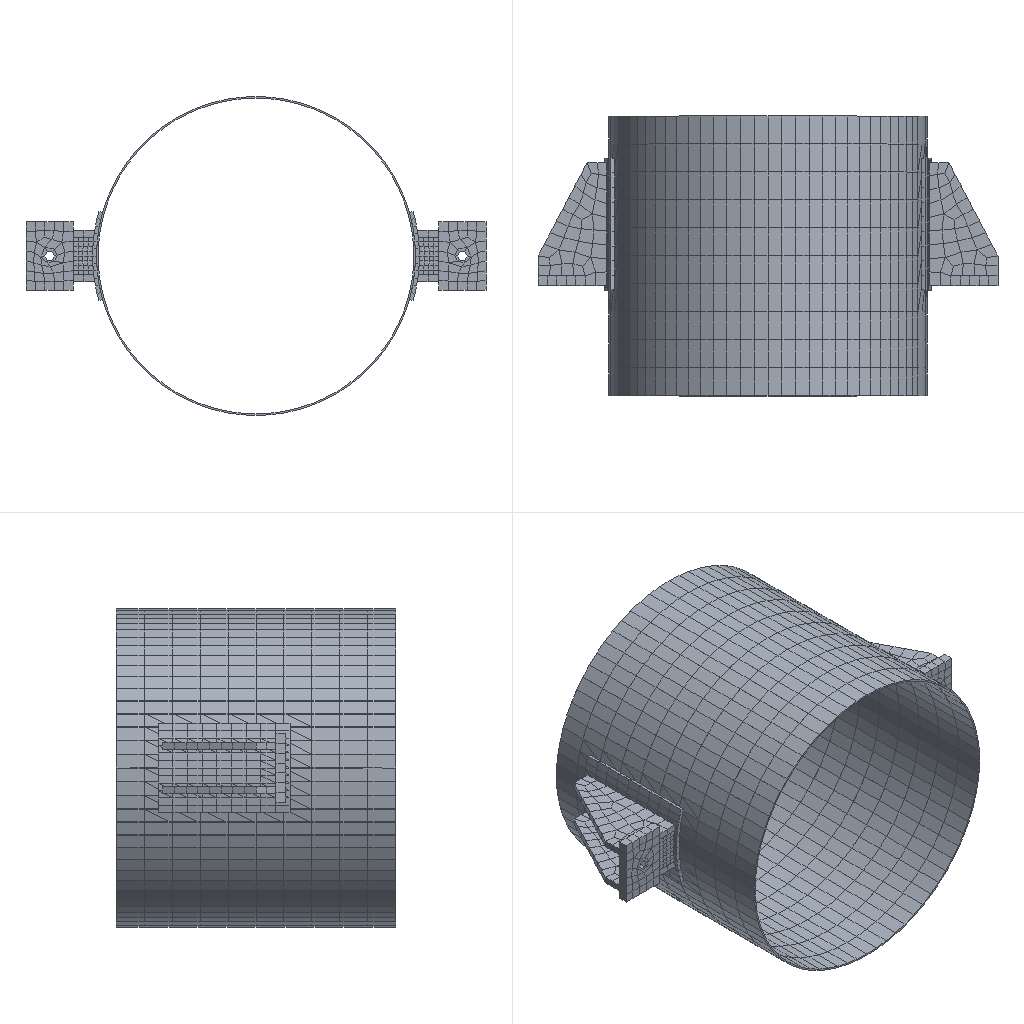Simulation study | ansys workbench
Ansys APDL input file, long lists of numbers shortened:
/batch
/config,noeldb,1     ! force off writing results to database
*get,_wallstrt,active,,time,wall
! ANSYS input file written by Workbench version 2022 R1
! File used for geometry attach:
/title,wbnew--____ (C5)
! ****** Begin Custom Load Command Snippet ******
/COM, ACT Extensions:
/COM,     LSDYNA, 2021.1
/COM,
! ****** End   Custom Load Command Snippet ******
*DIM,_wb_ProjectScratch_dir,string,248
_wb_ProjectScratch_dir(1) = ''
*DIM,_wb_SolverFiles_dir,string,248
_wb_SolverFiles_dir(1) = ''
*DIM,_wb_userfiles_dir,string,248
_wb_userfiles_dir(1) = ''
/com,--- Data in consistent NMM units. See Solving Units in the help system for more information.
/units,MPA
/nopr
/wb,file,start              !  signify a WB generated input file
/prep7
! Turn off shape checking because checks already performed inside WB mesher.
! See help system for more information.
SHPP,OFF,,NOWARN
/nolist
etcon,set             ! allow ANSYS to choose best KEYOP's for 180x elements, resets any applicable keyopt to MAPDL defaults
/com,*********** Nodes for the whole assembly ***********
nblock,3,,11156
(1i9,3e20.9e3)
        1    -9.929159159E+02     6.715040761E+02    -9.500000000E+01
! (10141 more lines like these left out)
-1
/wb,elem,start            !  set before creation of elements
/com,*********** Elements for Body 1 "__1^___1|__-__1" ***********
et,1,186
keyo,1,2,1          ! set full integration on SOLID186
eblock,19,solid,,720
(19i9)
        1        1        1        1        0        0        0        0       20        0      583     5200     5908     5907     5201     5204     5943     5942     5202
! (1439 more lines like these left out)
-1
/com,*********** Elements for Body 2 "__2^___1|__-__1" ***********
et,2,186
keyo,2,2,1          ! set full integration on SOLID186
eblock,19,solid,,108
(19i9)
        2        2        2        2        0        0        0        0       20        0      394     3257     3307     3371     3379     3293     3294     3370     3423
! (215 more lines like these left out)
-1
/com,*********** Elements for Body 3 "__3^___1|__-__1" ***********
et,3,186
keyo,3,2,1          ! set full integration on SOLID186
eblock,19,solid,,43
(19i9)
        3        3        3        3        0        0        0        0       20        0      103      797      820      801      798      844      821      840      843
! (85 more lines like these left out)
-1
/com,*********** Elements for Body 4 "__4^___1|__-__1" ***********
et,4,186
keyo,4,2,1          ! set full integration on SOLID186
eblock,19,solid,,38
(19i9)
        4        4        4        4        0        0        0        0       20        0      210     1631     1642     1646     1636     1662     1651     1647     1657
! (75 more lines like these left out)
-1
/com,*********** Elements for Body 5 "__4^___1|__-__1[2]" ***********
et,5,186
keyo,5,2,1          ! set full integration on SOLID186
eblock,19,solid,,38
(19i9)
        5        5        5        5        0        0        0        0       20        0      356     2834     2845     2849     2839     2865     2854     2850     2860
! (75 more lines like these left out)
-1
! (6 more sections like these left out)
/wb,elem,end               !  done creating elements
/com,*********** Send User Defined Coordinate System(s) ***********
csys,0
toffst,273.15,  ! Temperature offset from absolute zero
/com,*********** Set Reference Temperature ***********
tref,22.
/wb,mat,start              !  starting to send materials
/com,*********** Send Materials ***********
Temperature = 'TEMP' ! Temperature
MP,DENS,1,7.85e-09,	! tonne mm^-3
MP,ALPX,1,1.2e-05,	! C^-1
MP,C,1,434000000,	! mm^2 s^-2 C^-1
MP,KXX,1,60.5,	! tonne mm s^-3 C^-1
MP,RSVX,1,0.00017,	! ohm mm
MP,EX,1,200000,	! tonne s^-2 mm^-1
MP,NUXY,1,0.3,
MP,MURX,1,10000,
Temperature = 'TEMP' ! Temperature
MP,DENS,2,7.85e-09,	! tonne mm^-3
MP,ALPX,2,1.2e-05,	! C^-1
MP,C,2,434000000,	! mm^2 s^-2 C^-1
MP,KXX,2,60.5,	! tonne mm s^-3 C^-1
MP,RSVX,2,0.00017,	! ohm mm
MP,EX,2,200000,	! tonne s^-2 mm^-1
MP,NUXY,2,0.3,
MP,MURX,2,10000,
Temperature = 'TEMP' ! Temperature
MP,DENS,3,7.85e-09,	! tonne mm^-3
MP,ALPX,3,1.2e-05,	! C^-1
MP,C,3,434000000,	! mm^2 s^-2 C^-1
MP,KXX,3,60.5,	! tonne mm s^-3 C^-1
MP,RSVX,3,0.00017,	! ohm mm
MP,EX,3,200000,	! tonne s^-2 mm^-1
MP,NUXY,3,0.3,
MP,MURX,3,10000,
Temperature = 'TEMP' ! Temperature
MP,DENS,4,7.85e-09,	! tonne mm^-3
MP,ALPX,4,1.2e-05,	! C^-1
MP,C,4,434000000,	! mm^2 s^-2 C^-1
MP,KXX,4,60.5,	! tonne mm s^-3 C^-1
MP,RSVX,4,0.00017,	! ohm mm
MP,EX,4,200000,	! tonne s^-2 mm^-1
MP,NUXY,4,0.3,
MP,MURX,4,10000,
Temperature = 'TEMP' ! Temperature
MP,DENS,5,7.85e-09,	! tonne mm^-3
MP,ALPX,5,1.2e-05,	! C^-1
MP,C,5,434000000,	! mm^2 s^-2 C^-1
MP,KXX,5,60.5,	! tonne mm s^-3 C^-1
MP,RSVX,5,0.00017,	! ohm mm
MP,EX,5,200000,	! tonne s^-2 mm^-1
MP,NUXY,5,0.3,
MP,MURX,5,10000,
Temperature = 'TEMP' ! Temperature
MP,DENS,6,7.85e-09,	! tonne mm^-3
MP,ALPX,6,1.2e-05,	! C^-1
MP,C,6,434000000,	! mm^2 s^-2 C^-1
MP,KXX,6,60.5,	! tonne mm s^-3 C^-1
MP,RSVX,6,0.00017,	! ohm mm
MP,EX,6,200000,	! tonne s^-2 mm^-1
MP,NUXY,6,0.3,
MP,MURX,6,10000,
Temperature = 'TEMP' ! Temperature
MP,DENS,7,7.85e-09,	! tonne mm^-3
MP,ALPX,7,1.2e-05,	! C^-1
MP,C,7,434000000,	! mm^2 s^-2 C^-1
MP,KXX,7,60.5,	! tonne mm s^-3 C^-1
MP,RSVX,7,0.00017,	! ohm mm
MP,EX,7,200000,	! tonne s^-2 mm^-1
MP,NUXY,7,0.3,
MP,MURX,7,10000,
Temperature = 'TEMP' ! Temperature
MP,DENS,8,7.85e-09,	! tonne mm^-3
MP,ALPX,8,1.2e-05,	! C^-1
MP,C,8,434000000,	! mm^2 s^-2 C^-1
MP,KXX,8,60.5,	! tonne mm s^-3 C^-1
MP,RSVX,8,0.00017,	! ohm mm
MP,EX,8,200000,	! tonne s^-2 mm^-1
MP,NUXY,8,0.3,
MP,MURX,8,10000,
Temperature = 'TEMP' ! Temperature
MP,DENS,9,7.85e-09,	! tonne mm^-3
MP,ALPX,9,1.2e-05,	! C^-1
MP,C,9,434000000,	! mm^2 s^-2 C^-1
MP,KXX,9,60.5,	! tonne mm s^-3 C^-1
MP,RSVX,9,0.00017,	! ohm mm
MP,EX,9,200000,	! tonne s^-2 mm^-1
MP,NUXY,9,0.3,
MP,MURX,9,10000,
Temperature = 'TEMP' ! Temperature
MP,DENS,10,7.85e-09,	! tonne mm^-3
MP,ALPX,10,1.2e-05,	! C^-1
MP,C,10,434000000,	! mm^2 s^-2 C^-1
MP,KXX,10,60.5,	! tonne mm s^-3 C^-1
MP,RSVX,10,0.00017,	! ohm mm
MP,EX,10,200000,	! tonne s^-2 mm^-1
MP,NUXY,10,0.3,
MP,MURX,10,10000,
Temperature = 'TEMP' ! Temperature
MP,DENS,11,7.85e-09,	! tonne mm^-3
MP,ALPX,11,1.2e-05,	! C^-1
MP,C,11,434000000,	! mm^2 s^-2 C^-1
MP,KXX,11,60.5,	! tonne mm s^-3 C^-1
MP,RSVX,11,0.00017,	! ohm mm
MP,EX,11,200000,	! tonne s^-2 mm^-1
MP,NUXY,11,0.3,
MP,MURX,11,10000,
/wb,mat,end                !  done sending materials
!************************* Model Summary ********************
!__1^___1|__-__1,	Q355E,	matid,	1
!__2^___1|__-__1,	Q355E,	matid,	2
!__3^___1|__-__1,	Q355E,	matid,	3
!__4^___1|__-__1,	Q355E,	matid,	4
!__4^___1|__-__1[2],	Q355E,	matid,	5
!__5^___1|__-__1,	Q355E,	matid,	6
!__2^___1|__-__1[2],	Q355E,	matid,	7
!__4^___1|__-__1[3],	Q355E,	matid,	8
!__4^___1|__-__1[4],	Q355E,	matid,	9
!__3^___1|__-__1[2],	Q355E,	matid,	10
!__5^___1|__-__1[2],	Q355E,	matid,	11
!************************* End Model Summary ********************
! get the diagonal of the bounding box. Needed later for other things
*get,_xmin,node,,mnloc,x
*get,_ymin,node,,mnloc,y
*get,_zmin,node,,mnloc,z
*get,_xmax,node,,mxloc,x
*get,_ymax,node,,mxloc,y
*get,_zmax,node,,mxloc,z
_ASMDIAG=(_xmax-_xmin)*(_xmax-_xmin)+(_ymax-_ymin)*(_ymax-_ymin)+(_zmax-_zmin)*(_zmax-_zmin)
_ASMDIAG=SQRT(_ASMDIAG)
/wb,contact,start          !  starting to send contact
/com,*********** Create Contact "接触区域" ***********
/com,            Real Constant Set For Above Contact Is 13 & 12
*set,tid,13
*set,cid,12
r,tid
r,cid
et,tid,170
et,cid,174
eblock,10,,,48
(15i9)
     4275       13       13       13        0     5305     5306     5271     5270     7916     7814     7810     7811
! (47 more lines like these left out)
-1
eblock,10,,,48
(15i9)
     4323       12       12       12        0     5305     5306     5271     5270     7916     7814     7810     7811
! (47 more lines like these left out)
-1
eblock,10,,,108
(15i9)
     4371       12       13       12        0     3308     3253     3298     3299     3672     3671     3808     3810
! (107 more lines like these left out)
-1
eblock,10,,,108
(15i9)
     4479       13       12       13        0     3308     3253     3298     3299     3672     3671     3808     3810
! (107 more lines like these left out)
-1
keyo,cid,8,2               ! auto create asymmetric contact (from Program Controlled setting)
keyo,cid,10,0              ! adjust contact stiffness each NR iteration (from Program Controlled setting)
keyo,cid,12,5              ! bonded always
keyo,cid,18,1              ! small sliding turned on by application
keyo,cid,2,0               ! augmented Lagrange (from Program Controlled setting)
keyo,cid,4,0               ! on Gauss point (from Program Controlled setting)
keyo,cid,9,1               ! ignore initial gaps/penetration
keyo,cid,7,0               ! No Prediction
rmod,tid,3,10.      ! FKN
rmod,tid,5,0.       ! ICONT
rmod,tid,6,0.       ! PINB
rmod,tid,10,0.      ! CNOF
rmod,tid,12,0.      ! FKT
rmod,tid,36,56      ! WB DSID
rmod,cid,3,10.      ! FKN
rmod,cid,5,0.       ! ICONT
rmod,cid,6,0.       ! PINB
rmod,cid,10,0.      ! CNOF
rmod,cid,12,0.      ! FKT
rmod,cid,36,56      ! WB DSID
/com,*********** Create Contact "接触区域 2" ***********
/com,            Real Constant Set For Above Contact Is 15 & 14
*set,tid,15
*set,cid,14
r,tid
r,cid
et,tid,170
et,cid,174
eblock,10,,,48
(15i9)
     4587       15       15       15        0     5675     5676     5641     5640     8928     8862     8859     8860
! (47 more lines like these left out)
-1
eblock,10,,,48
(15i9)
     4635       14       14       14        0     5675     5676     5641     5640     8928     8862     8859     8860
! (47 more lines like these left out)
-1
eblock,10,,,108
(15i9)
     4683       14       15       14        0     2105     2050     2095     2096     2469     2468     2605     2607
! (107 more lines like these left out)
-1
eblock,10,,,108
(15i9)
     4791       15       14       15        0     2105     2050     2095     2096     2469     2468     2605     2607
! (107 more lines like these left out)
-1
keyo,cid,8,2               ! auto create asymmetric contact (from Program Controlled setting)
keyo,cid,10,0              ! adjust contact stiffness each NR iteration (from Program Controlled setting)
keyo,cid,12,5              ! bonded always
keyo,cid,18,1              ! small sliding turned on by application
keyo,cid,2,0               ! augmented Lagrange (from Program Controlled setting)
keyo,cid,4,0               ! on Gauss point (from Program Controlled setting)
keyo,cid,9,1               ! ignore initial gaps/penetration
keyo,cid,7,0               ! No Prediction
rmod,tid,3,10.      ! FKN
rmod,tid,5,0.       ! ICONT
rmod,tid,6,0.       ! PINB
rmod,tid,10,0.      ! CNOF
rmod,tid,12,0.      ! FKT
rmod,tid,36,59      ! WB DSID
rmod,cid,3,10.      ! FKN
rmod,cid,5,0.       ! ICONT
rmod,cid,6,0.       ! PINB
rmod,cid,10,0.      ! CNOF
rmod,cid,12,0.      ! FKT
rmod,cid,36,59      ! WB DSID
/com,*********** Create Contact "接触区域 3" ***********
/com,            Real Constant Set For Above Contact Is 17 & 16
*set,tid,17
*set,cid,16
r,tid
r,cid
et,tid,170
et,cid,174
eblock,10,,,18
(15i9)
     4899       17       17       17        0     3191     3192     3233     3234     3492     3498     3622     3494
! (17 more lines like these left out)
-1
eblock,10,,,18
(15i9)
     4917       16       16       16        0     3191     3192     3233     3234     3492     3498     3622     3494
! (17 more lines like these left out)
-1
eblock,10,,,9
(15i9)
     4935       16       17       16        0     1719     1720     1679     1680     1953     1893     1892     1895
! (8 more lines like these left out)
-1
eblock,10,,,9
(15i9)
     4944       17       16       17        0     1719     1720     1679     1680     1953     1893     1892     1895
! (8 more lines like these left out)
-1
keyo,cid,8,2               ! auto create asymmetric contact (from Program Controlled setting)
keyo,cid,10,0              ! adjust contact stiffness each NR iteration (from Program Controlled setting)
keyo,cid,12,5              ! bonded always
keyo,cid,18,1              ! small sliding turned on by application
keyo,cid,2,0               ! augmented Lagrange (from Program Controlled setting)
keyo,cid,4,0               ! on Gauss point (from Program Controlled setting)
keyo,cid,9,1               ! ignore initial gaps/penetration
keyo,cid,7,0               ! No Prediction
rmod,tid,3,10.      ! FKN
rmod,tid,5,0.       ! ICONT
rmod,tid,6,0.       ! PINB
rmod,tid,10,0.      ! CNOF
rmod,tid,12,0.      ! FKT
rmod,tid,36,62      ! WB DSID
rmod,cid,3,10.      ! FKN
rmod,cid,5,0.       ! ICONT
rmod,cid,6,0.       ! PINB
rmod,cid,10,0.      ! CNOF
rmod,cid,12,0.      ! FKT
rmod,cid,36,62      ! WB DSID
/com,*********** Create Contact "接触区域 4" ***********
/com,            Real Constant Set For Above Contact Is 19 & 18
*set,tid,19
*set,cid,18
r,tid
r,cid
et,tid,170
et,cid,174
eblock,10,,,18
(15i9)
     4953       19       19       19        0     3380     3381     3421     3422     3955     3960     4026     3957
! (17 more lines like these left out)
-1
eblock,10,,,18
(15i9)
     4971       18       18       18        0     3380     3381     3421     3422     3955     3960     4026     3957
! (17 more lines like these left out)
-1
eblock,10,,,9
(15i9)
     4989       18       19       18        0     2922     2923     2882     2883     3156     3096     3095     3098
! (8 more lines like these left out)
-1
eblock,10,,,9
(15i9)
     4998       19       18       19        0     2922     2923     2882     2883     3156     3096     3095     3098
! (8 more lines like these left out)
-1
keyo,cid,8,2               ! auto create asymmetric contact (from Program Controlled setting)
keyo,cid,10,0              ! adjust contact stiffness each NR iteration (from Program Controlled setting)
keyo,cid,12,5              ! bonded always
keyo,cid,18,1              ! small sliding turned on by application
keyo,cid,2,0               ! augmented Lagrange (from Program Controlled setting)
keyo,cid,4,0               ! on Gauss point (from Program Controlled setting)
keyo,cid,9,1               ! ignore initial gaps/penetration
keyo,cid,7,0               ! No Prediction
rmod,tid,3,10.      ! FKN
rmod,tid,5,0.       ! ICONT
rmod,tid,6,0.       ! PINB
rmod,tid,10,0.      ! CNOF
rmod,tid,12,0.      ! FKT
rmod,tid,36,65      ! WB DSID
rmod,cid,3,10.      ! FKN
rmod,cid,5,0.       ! ICONT
rmod,cid,6,0.       ! PINB
rmod,cid,10,0.      ! CNOF
rmod,cid,12,0.      ! FKT
rmod,cid,36,65      ! WB DSID
/com,*********** Create Contact "接触区域 5" ***********
/com,            Real Constant Set For Above Contact Is 21 & 20
*set,tid,21
*set,cid,20
r,tid
r,cid
et,tid,170
et,cid,174
eblock,10,,,12
(15i9)
     5007       21       21       21        0     3245     3190     3235     3236     3490     3489     3626     3628
! (11 more lines like these left out)
-1
eblock,10,,,12
(15i9)
     5019       20       20       20        0     3245     3190     3235     3236     3490     3489     3626     3628
! (11 more lines like these left out)
-1
eblock,10,,,16
(15i9)
     5031       20       21       20        0     1273     1298     1234     1250     1580     1508     1507     1540
! (15 more lines like these left out)
-1
eblock,10,,,16
(15i9)
     5047       21       20       21        0     1273     1298     1234     1250     1580     1508     1507     1540
! (15 more lines like these left out)
-1
keyo,cid,8,2               ! auto create asymmetric contact (from Program Controlled setting)
keyo,cid,10,0              ! adjust contact stiffness each NR iteration (from Program Controlled setting)
keyo,cid,12,5              ! bonded always
keyo,cid,18,1              ! small sliding turned on by application
keyo,cid,2,0               ! augmented Lagrange (from Program Controlled setting)
keyo,cid,4,0               ! on Gauss point (from Program Controlled setting)
keyo,cid,9,1               ! ignore initial gaps/penetration
keyo,cid,7,0               ! No Prediction
rmod,tid,3,10.      ! FKN
rmod,tid,5,0.       ! ICONT
rmod,tid,6,0.       ! PINB
rmod,tid,10,0.      ! CNOF
rmod,tid,12,0.      ! FKT
rmod,tid,36,68      ! WB DSID
rmod,cid,3,10.      ! FKN
rmod,cid,5,0.       ! ICONT
rmod,cid,6,0.       ! PINB
rmod,cid,10,0.      ! CNOF
rmod,cid,12,0.      ! FKT
rmod,cid,36,68      ! WB DSID
! (13 more sections like these left out)
/wb,contact,end            !  done creating contacts
/golist
/wb,load,start             !  starting to send loads
/com,*********** Fixed Supports ***********
CMBLOCK,_FIXEDSU,NODE,       60
(8i10)
       849       850       875       876       877       878       879       880
! (7 more lines like these left out)
cmsel,s,_FIXEDSU
d,all,all
nsel,all
/com,*********** Define Force Using Surface Effect Elements ***********
local,12,0,0.,0.,0.,0.,0.,0.
csys,0
et,48,154
eblock,10,,,86
(15i9)
     5571       48       48       48       12     4075     4078     4079     4056     4297     4302     4246     4244
! (85 more lines like these left out)
-1
esel,s,type,,48
keyop,48,2,1                ! Apply load in local coordinate system
keyop,48,7,1                ! Use original area so load is constant in large deformation
esel,all
/gst,on,on
fini
*get,_numnode,node,0,count
*get,_numelem,elem,0,count
*get, _MAXELEMNUM, elem, 0, NUM, MAX
*get, _MAXNODENUM, node, 0, NUM, MAX
*get, _MAXELEMTYPE, etyp, 0, NUM, MAX
*get, _MAXREALCONST, real, 0, NUM, MAX
/go
/wb,load,end               !  done creating loads
/com,--- Number of total nodes = %_numnode%
/com,--- Number of contact elements = 1382
/com,--- Number of spring elements = 0
/com,--- Number of bearing elements = 0
/com,--- Number of solid elements = 1302
/com,--- Number of condensed parts = 0
/com,--- Number of total elements = %_numelem%
*get,_wallbsol,active,,time,wall
/com,****************************************************************************
/com,*************************    SOLUTION       ********************************
/com,****************************************************************************
/solu
antype,0                   ! static analysis
_thickRatio=  0     ! Ratio of thick parts in the model
eqsl,sparse,,,,,1
cntr,print,1               ! print out contact info and also make no initial contact an error
dmpoption,emat,no             ! Don't combine emat file for DANSYS
dmpoption,esav,no             ! Don't combine esav file for DANSYS
nldiag,cont,iter           ! print out contact info each equilibrium iteration
rescontrol,,none                 ! Do not keep any restart files
/com,****************************************************
/com,******************* SOLVE FOR LS 1 OF 1 ****************
esel,s,type,,48
nsle
sfe,all,1,pres,1,0.
sfe,all,2,pres,1,3.65
sfe,all,3,pres,1,0.
nsel,all
esel,all
/nopr
/gopr
nsub,1,1,1
time,1.
outres,erase
outres,all,none
outres,nsol,all,
outres,rsol,all
outres,eangl,all
outres,etmp,all
outres,veng,all
outres,strs,all,
outres,epel,all,
outres,eppl,all,
outres,cont,all,
! *********** WB SOLVE COMMAND ***********
! check interactive state
*get,ANSINTER_,active,,int
*if,ANSINTER_,ne,0,then
/eof
*endif
solve
/com *************** Write FE CONNECTORS *********
CEWRITE,file,ce,,INTE
/com,****************************************************
/com,*************** FINISHED SOLVE FOR LS 1 *************
*get,_wallasol,active,,time,wall
/nopr
*get,_numnode,node,0,count
*get,_numelem,elem,0,count
*get, _MAXELEMNUM, elem, 0, NUM, MAX
*get, _MAXNODENUM, node, 0, NUM, MAX,,,INTERNAL
*get, _MAXELEMTYPE, etyp, 0, NUM, MAX
*get, _MAXREALCONST, real, 0, NUM, MAX
/gopr
/post1
xmlo,ENCODING,ISO-8859-1
xmlo,parm
/xml,parm,xml
fini
/gopr
*get,_walldone,active,,time,wall
_preptime=(_wallbsol-_wallstrt)*3600
_solvtime=(_wallasol-_wallbsol)*3600
_posttime=(_walldone-_wallasol)*3600
_totaltim=(_walldone-_wallstrt)*3600
*get,_dlbratio,active,0,solu,dlbr
*get,_combtime,active,0,solu,comb
*get,_ssmode,active,0,solu,ssmm
*get,_ndofs,active,0,solu,ndof
*get,_sol_end_time,active,0,set,time
*if,_sol_end_time,eq,1.,then
/fclean				!clean distributed files
*endif
/com,--- Total number of nodes = %_numnode%
/com,--- Total number of elements = %_numelem%
/com,--- Element load balance ratio = %_dlbratio%
/com,--- Time to combine distributed files = %_combtime%
/com,--- Sparse memory mode = %_ssmode%
/com,--- Number of DOF = %_ndofs%
/wb,file,end               ! done with WB generated input